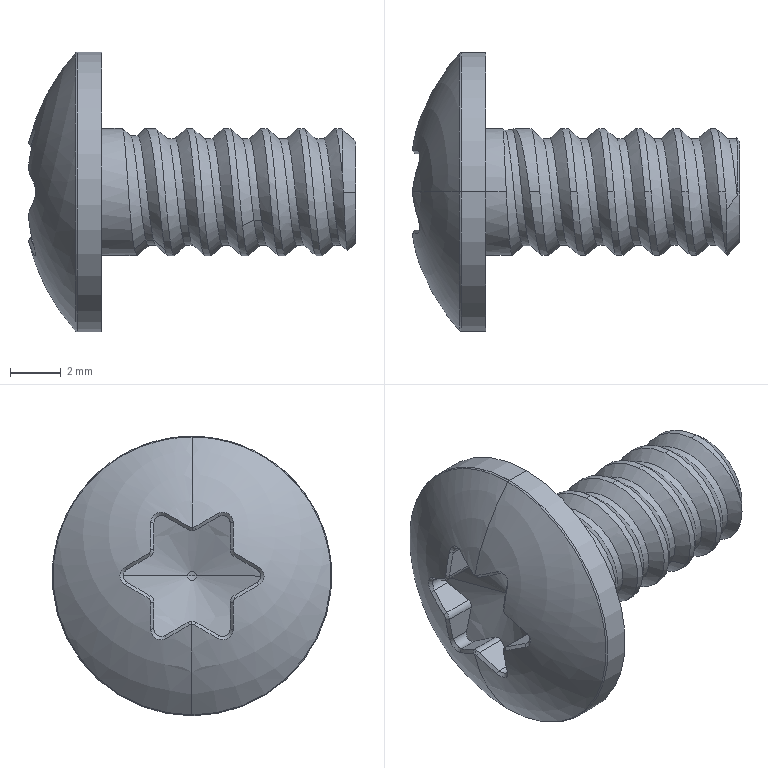Part | SolidWorks | features BaseBody 1 | 1 solid | 87 faces | box 12.881 x 11 x 11.001 mm | volume 345.929 mm3 | cylinder 27 | spline 23 | cone 17 | plane 14 | sphere 4 | torus 2 | commonest cylinder face diameters 5 x13 0.6 x12 11 x2